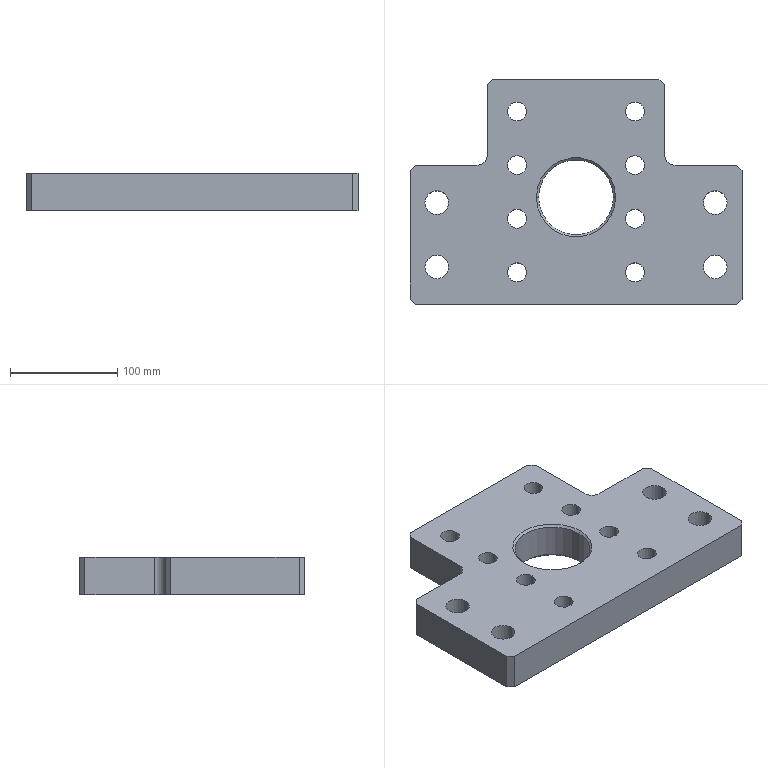Part | SolidWorks | features ICE 5, Chamfer 3, Fillet 2, HoleWzd 2, Extrusion 1 | 1 solid | 72 faces | box 310 x 210 x 35 mm | volume 1574562 mm3 | cylinder 44 | plane 24 | cone 4 | commonest cylinder face diameters 17.5 x16 26 x16 22 x8 20 x2 70 x2